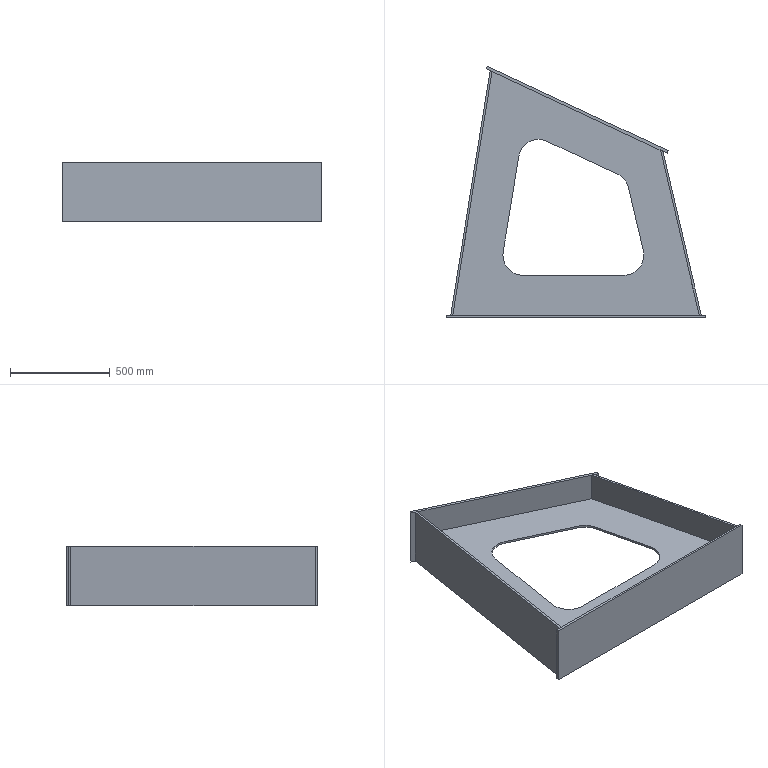Part | STEP file | Motor bracket leg_Default<As machined> | 5 solids | 39 faces | box 1300 x 1259 x 300 mm | volume 22043993 mm3 | plane 34 | cylinder 5 | commonest cylinder face diameters 200 x5